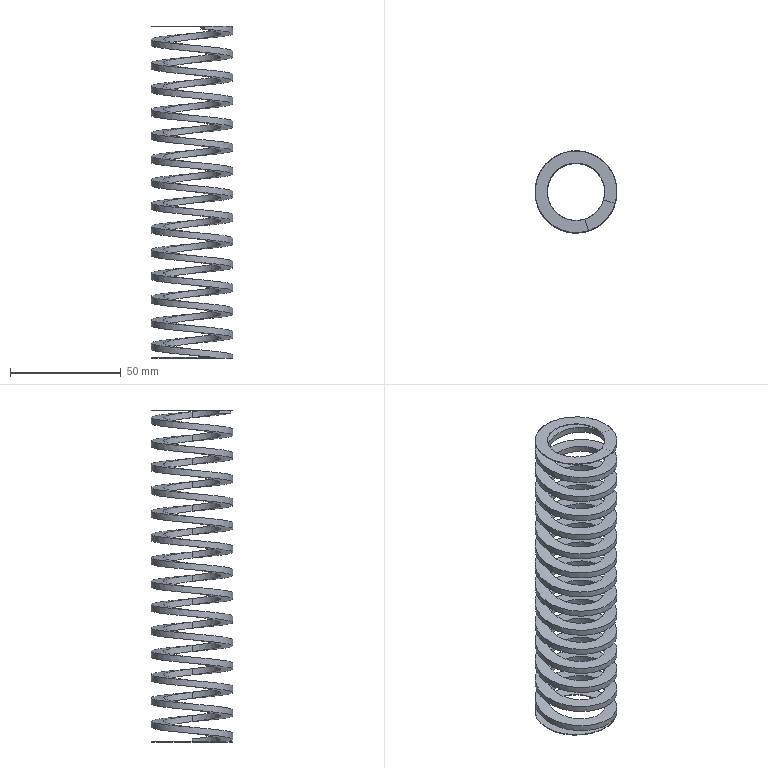Part | STEP file | 1_id654_xmt_txt | 1 solid | 38 faces | box 37 x 37 x 150 mm | volume 21369 mm3 | cylinder 30 | plane 6 | spline 2 | commonest cylinder face diameters 26 x15 37 x15